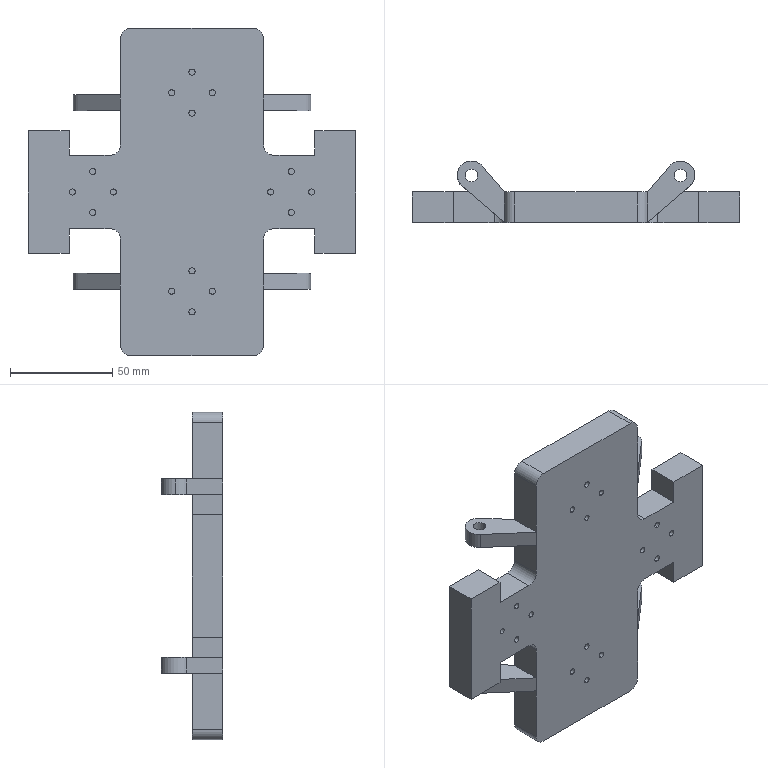Part | SolidWorks | features ICE 6, Fillet 2, MirrorPattern 2, Extrusion 1 | 1 solid | 112 faces | box 160 x 30.068 x 160 mm | volume 240546 mm3 | plane 58 | cylinder 54 | commonest cylinder face diameters 3 x32 6.2 x8 10 x8 14 x6